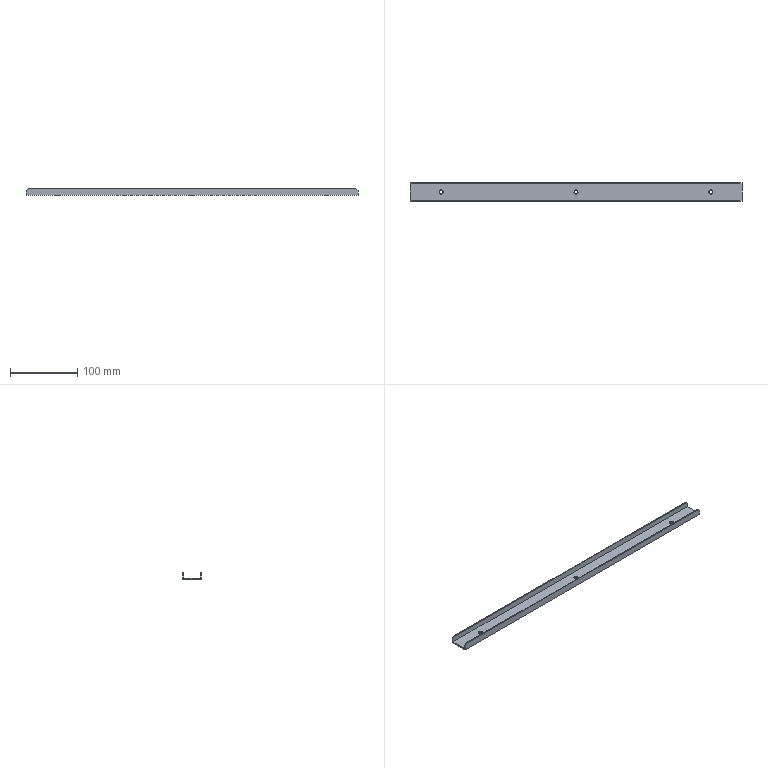Part | STEP file | 1 solid | 20 faces | box 492 x 27 x 10 mm | volume 32318 mm3 | plane 14 | cylinder 6 | commonest cylinder face diameters 6 x6